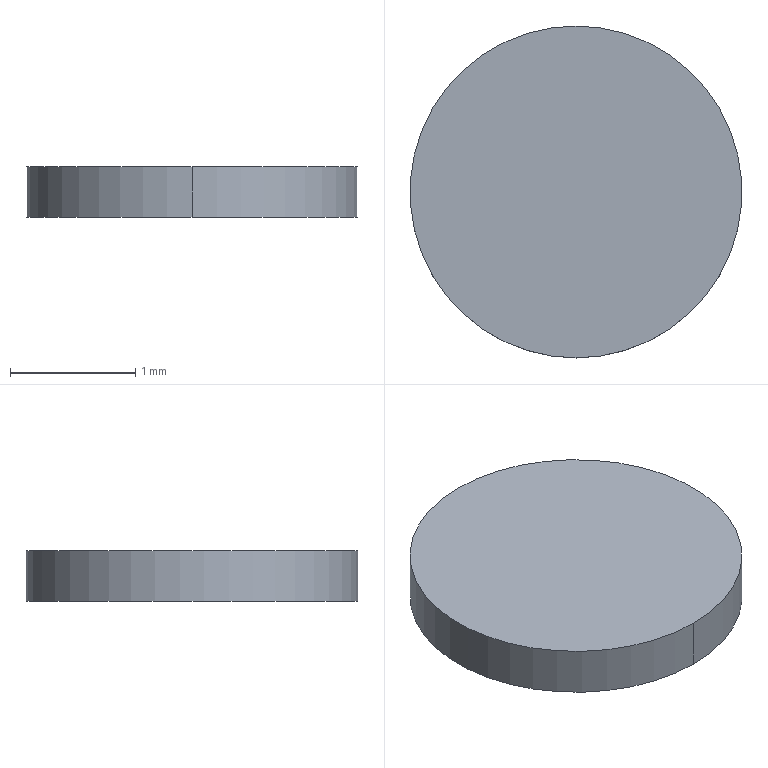Part | STEP file | LRS-150-12_X2_5F00517375-151328 | 1 solid | 4 faces | box 2.65 x 2.65 x 0.4 mm | volume 2.206 mm3 | cylinder 2 | plane 2 | commonest cylinder face diameters 2.65 x2
STEP:
#1=CARTESIAN_POINT('',(0.,0.,0.));
#2=DIRECTION('',(0.,0.,1.));
#3=DIRECTION('',(1.,0.,0.));
#4=AXIS2_PLACEMENT_3D('',#1,#2,#3);
#5=CARTESIAN_POINT('',(-275.667,233.7,-4.8));
#6=VERTEX_POINT('',#5);
#7=CARTESIAN_POINT('',(-275.667,233.7,-4.4));
#8=VERTEX_POINT('',#7);
#9=CARTESIAN_POINT('',(-275.667,233.7,-4.8));
#10=DIRECTION('',(0.,0.,1.));
#11=VECTOR('',#10,1.);
#12=LINE('',#9,#11);
#13=CARTESIAN_POINT('',(-275.667,235.025,-5.145));
#14=DIRECTION('',(0.,0.,-1.));
#15=DIRECTION('',(0.,-1.,0.));
#16=AXIS2_PLACEMENT_3D('',#13,#14,#15);
#17=CYLINDRICAL_SURFACE('',#16,1.325);
#18=CARTESIAN_POINT('',(6.283,-0.345));
#19=DIRECTION('',(0.,-1.));
#20=VECTOR('',#19,1.);
#21=LINE('',#18,#20);
#22=(GEOMETRIC_REPRESENTATION_CONTEXT(2)PARAMETRIC_REPRESENTATION_CONTEXT()REPRESENTATION_CONTEXT('',''));
#23=DEFINITIONAL_REPRESENTATION('',(#21),#22);
#24=PCURVE('',#17,#23);
#25=CARTESIAN_POINT('',(-275.667,235.025,-5.145));
#26=DIRECTION('',(0.,0.,-1.));
#27=DIRECTION('',(0.,-1.,0.));
#28=AXIS2_PLACEMENT_3D('',#25,#26,#27);
#29=CYLINDRICAL_SURFACE('',#28,1.325);
#30=CARTESIAN_POINT('',(0.,-0.345));
#31=DIRECTION('',(0.,-1.));
#32=VECTOR('',#31,1.);
#33=LINE('',#30,#32);
#34=(GEOMETRIC_REPRESENTATION_CONTEXT(2)PARAMETRIC_REPRESENTATION_CONTEXT()REPRESENTATION_CONTEXT('',''));
#35=DEFINITIONAL_REPRESENTATION('',(#33),#34);
#36=PCURVE('',#29,#35);
#37=SURFACE_CURVE('',#12,(#24,#36),.PCURVE_S1.);
#38=EDGE_CURVE('',#6,#8,#37,.T.);
#39=ORIENTED_EDGE('',*,*,#38,.F.);
#40=CARTESIAN_POINT('',(-275.667,236.35,-4.8));
#41=VERTEX_POINT('',#40);
#42=CARTESIAN_POINT('',(-275.667,235.025,-4.8));
#43=DIRECTION('',(0.,0.,-1.));
#44=DIRECTION('',(0.,1.,0.));
#45=AXIS2_PLACEMENT_3D('',#42,#43,#44);
#46=CIRCLE('',#45,1.325);
#47=CARTESIAN_POINT('',(3.142,-0.345));
#48=DIRECTION('',(1.,0.));
#49=VECTOR('',#48,1.);
#50=LINE('',#47,#49);
#51=(GEOMETRIC_REPRESENTATION_CONTEXT(2)PARAMETRIC_REPRESENTATION_CONTEXT()REPRESENTATION_CONTEXT('',''));
#52=DEFINITIONAL_REPRESENTATION('',(#50),#51);
#53=PCURVE('',#17,#52);
#54=CARTESIAN_POINT('',(-217.675,251.825,-4.8));
#55=DIRECTION('',(0.,0.,-1.));
#56=DIRECTION('',(1.,0.,0.));
#57=AXIS2_PLACEMENT_3D('',#54,#55,#56);
#58=PLANE('',#57);
#59=CARTESIAN_POINT('',(-57.991,16.8));
#60=DIRECTION('',(0.,-1.));
#61=AXIS2_PLACEMENT_2D('',#59,#60);
#62=CIRCLE('',#61,1.325);
#63=(GEOMETRIC_REPRESENTATION_CONTEXT(2)PARAMETRIC_REPRESENTATION_CONTEXT()REPRESENTATION_CONTEXT('',''));
#64=DEFINITIONAL_REPRESENTATION('',(#62),#63);
#65=PCURVE('',#58,#64);
#66=SURFACE_CURVE('',#46,(#53,#65),.PCURVE_S1.);
#67=EDGE_CURVE('',#41,#6,#66,.T.);
#68=ORIENTED_EDGE('',*,*,#67,.F.);
#69=CARTESIAN_POINT('',(-275.667,236.35,-4.4));
#70=VERTEX_POINT('',#69);
#71=CARTESIAN_POINT('',(-275.667,236.35,-4.8));
#72=DIRECTION('',(0.,0.,1.));
#73=VECTOR('',#72,1.);
#74=LINE('',#71,#73);
#75=CARTESIAN_POINT('',(3.142,-0.345));
#76=DIRECTION('',(0.,-1.));
#77=VECTOR('',#76,1.);
#78=LINE('',#75,#77);
#79=(GEOMETRIC_REPRESENTATION_CONTEXT(2)PARAMETRIC_REPRESENTATION_CONTEXT()REPRESENTATION_CONTEXT('',''));
#80=DEFINITIONAL_REPRESENTATION('',(#78),#79);
#81=PCURVE('',#17,#80);
#82=CARTESIAN_POINT('',(3.142,-0.345));
#83=DIRECTION('',(0.,-1.));
#84=VECTOR('',#83,1.);
#85=LINE('',#82,#84);
#86=(GEOMETRIC_REPRESENTATION_CONTEXT(2)PARAMETRIC_REPRESENTATION_CONTEXT()REPRESENTATION_CONTEXT('',''));
#87=DEFINITIONAL_REPRESENTATION('',(#85),#86);
#88=PCURVE('',#29,#87);
#89=SURFACE_CURVE('',#74,(#81,#88),.PCURVE_S1.);
#90=EDGE_CURVE('',#41,#70,#89,.T.);
#91=ORIENTED_EDGE('',*,*,#90,.T.);
#92=CARTESIAN_POINT('',(-275.667,235.025,-4.4));
#93=DIRECTION('',(0.,0.,1.));
#94=DIRECTION('',(0.,-1.,0.));
#95=AXIS2_PLACEMENT_3D('',#92,#93,#94);
#96=CIRCLE('',#95,1.325);
#97=CARTESIAN_POINT('',(6.283,-0.745));
#98=DIRECTION('',(-1.,0.));
#99=VECTOR('',#98,1.);
#100=LINE('',#97,#99);
#101=(GEOMETRIC_REPRESENTATION_CONTEXT(2)PARAMETRIC_REPRESENTATION_CONTEXT()REPRESENTATION_CONTEXT('',''));
#102=DEFINITIONAL_REPRESENTATION('',(#100),#101);
#103=PCURVE('',#17,#102);
#104=CARTESIAN_POINT('',(-217.675,251.825,-4.4));
#105=DIRECTION('',(0.,0.,-1.));
#106=DIRECTION('',(1.,0.,0.));
#107=AXIS2_PLACEMENT_3D('',#104,#105,#106);
#108=PLANE('',#107);
#109=CARTESIAN_POINT('',(-57.991,18.125));
#110=CARTESIAN_POINT('',(-55.696,18.125));
#111=CARTESIAN_POINT('',(-56.844,16.137));
#112=CARTESIAN_POINT('',(-57.991,14.15));
#113=CARTESIAN_POINT('',(-59.139,16.137));
#114=CARTESIAN_POINT('',(-60.286,18.125));
#115=CARTESIAN_POINT('',(-57.991,18.125));
#116=(BOUNDED_CURVE()B_SPLINE_CURVE(2,(#109,#110,#111,#112,#113,#114,#115),.UNSPECIFIED.,.T.,.F.)B_SPLINE_CURVE_WITH_KNOTS((1,2,2,2,2,1),(-2.094,0.,2.094,4.189,6.283,8.378),.UNSPECIFIED.)CURVE()GEOMETRIC_REPRESENTATION_ITEM()RATIONAL_B_SPLINE_CURVE((1.,0.5,1.,0.5,1.,0.5,1.))REPRESENTATION_ITEM(''));
#117=(GEOMETRIC_REPRESENTATION_CONTEXT(2)PARAMETRIC_REPRESENTATION_CONTEXT()REPRESENTATION_CONTEXT('',''));
#118=DEFINITIONAL_REPRESENTATION('',(#116),#117);
#119=PCURVE('',#108,#118);
#120=SURFACE_CURVE('',#96,(#103,#119),.PCURVE_S1.);
#121=EDGE_CURVE('',#8,#70,#120,.T.);
#122=ORIENTED_EDGE('',*,*,#121,.F.);
#123=EDGE_LOOP('',(#39,#68,#91,#122));
#124=FACE_BOUND('',#123,.T.);
#125=ADVANCED_FACE('',(#124),#17,.T.);
#126=ORIENTED_EDGE('',*,*,#121,.F.);
#127=CARTESIAN_POINT('',(-275.667,235.025,-4.4));
#128=DIRECTION('',(0.,0.,1.));
#129=DIRECTION('',(0.,1.,0.));
#130=AXIS2_PLACEMENT_3D('',#127,#128,#129);
#131=CIRCLE('',#130,1.325);
#132=CARTESIAN_POINT('',(-57.991,15.475));
#133=CARTESIAN_POINT('',(-60.286,15.475));
#134=CARTESIAN_POINT('',(-59.139,17.462));
#135=CARTESIAN_POINT('',(-57.991,19.45));
#136=CARTESIAN_POINT('',(-56.844,17.462));
#137=CARTESIAN_POINT('',(-55.696,15.475));
#138=CARTESIAN_POINT('',(-57.991,15.475));
#139=(BOUNDED_CURVE()B_SPLINE_CURVE(2,(#132,#133,#134,#135,#136,#137,#138),.UNSPECIFIED.,.T.,.F.)B_SPLINE_CURVE_WITH_KNOTS((1,2,2,2,2,1),(-2.094,0.,2.094,4.189,6.283,8.378),.UNSPECIFIED.)CURVE()GEOMETRIC_REPRESENTATION_ITEM()RATIONAL_B_SPLINE_CURVE((1.,0.5,1.,0.5,1.,0.5,1.))REPRESENTATION_ITEM(''));
#140=(GEOMETRIC_REPRESENTATION_CONTEXT(2)PARAMETRIC_REPRESENTATION_CONTEXT()REPRESENTATION_CONTEXT('',''));
#141=DEFINITIONAL_REPRESENTATION('',(#139),#140);
#142=PCURVE('',#108,#141);
#143=CARTESIAN_POINT('',(3.142,-0.745));
#144=DIRECTION('',(-1.,0.));
#145=VECTOR('',#144,1.);
#146=LINE('',#143,#145);
#147=(GEOMETRIC_REPRESENTATION_CONTEXT(2)PARAMETRIC_REPRESENTATION_CONTEXT()REPRESENTATION_CONTEXT('',''));
#148=DEFINITIONAL_REPRESENTATION('',(#146),#147);
#149=PCURVE('',#29,#148);
#150=SURFACE_CURVE('',#131,(#142,#149),.PCURVE_S1.);
#151=EDGE_CURVE('',#70,#8,#150,.T.);
#152=ORIENTED_EDGE('',*,*,#151,.F.);
#153=EDGE_LOOP('',(#126,#152));
#154=FACE_BOUND('',#153,.F.);
#155=ADVANCED_FACE('',(#154),#108,.F.);
#156=CARTESIAN_POINT('',(-275.667,235.025,-4.8));
#157=DIRECTION('',(0.,0.,-1.));
#158=DIRECTION('',(0.,-1.,0.));
#159=AXIS2_PLACEMENT_3D('',#156,#157,#158);
#160=CIRCLE('',#159,1.325);
#161=CARTESIAN_POINT('',(0.,-0.345));
#162=DIRECTION('',(1.,0.));
#163=VECTOR('',#162,1.);
#164=LINE('',#161,#163);
#165=(GEOMETRIC_REPRESENTATION_CONTEXT(2)PARAMETRIC_REPRESENTATION_CONTEXT()REPRESENTATION_CONTEXT('',''));
#166=DEFINITIONAL_REPRESENTATION('',(#164),#165);
#167=PCURVE('',#29,#166);
#168=CARTESIAN_POINT('',(-57.991,16.8));
#169=DIRECTION('',(0.,1.));
#170=AXIS2_PLACEMENT_2D('',#168,#169);
#171=CIRCLE('',#170,1.325);
#172=(GEOMETRIC_REPRESENTATION_CONTEXT(2)PARAMETRIC_REPRESENTATION_CONTEXT()REPRESENTATION_CONTEXT('',''));
#173=DEFINITIONAL_REPRESENTATION('',(#171),#172);
#174=PCURVE('',#58,#173);
#175=SURFACE_CURVE('',#160,(#167,#174),.PCURVE_S1.);
#176=EDGE_CURVE('',#6,#41,#175,.T.);
#177=ORIENTED_EDGE('',*,*,#176,.F.);
#178=ORIENTED_EDGE('',*,*,#38,.T.);
#179=ORIENTED_EDGE('',*,*,#151,.F.);
#180=ORIENTED_EDGE('',*,*,#90,.F.);
#181=EDGE_LOOP('',(#177,#178,#179,#180));
#182=FACE_BOUND('',#181,.T.);
#183=ADVANCED_FACE('',(#182),#29,.T.);
#184=ORIENTED_EDGE('',*,*,#67,.F.);
#185=ORIENTED_EDGE('',*,*,#176,.F.);
#186=EDGE_LOOP('',(#184,#185));
#187=FACE_BOUND('',#186,.F.);
#188=ADVANCED_FACE('',(#187),#58,.T.);
#189=CLOSED_SHELL('',(#125,#155,#183,#188));
#190=MANIFOLD_SOLID_BREP('',#189);
#191=(LENGTH_UNIT()NAMED_UNIT(*)SI_UNIT(.MILLI.,.METRE.));
#192=UNCERTAINTY_MEASURE_WITH_UNIT(LENGTH_MEASURE(0.0000001),#191,'','');
#193=(NAMED_UNIT(*)PLANE_ANGLE_UNIT()SI_UNIT($,.RADIAN.));
#194=(NAMED_UNIT(*)SI_UNIT($,.STERADIAN.)SOLID_ANGLE_UNIT());
#195=(GEOMETRIC_REPRESENTATION_CONTEXT(3)GLOBAL_UNCERTAINTY_ASSIGNED_CONTEXT((#192))GLOBAL_UNIT_ASSIGNED_CONTEXT((#191,#193,#194))REPRESENTATION_CONTEXT('',''));
#196=ADVANCED_BREP_SHAPE_REPRESENTATION('',(#4,#190),#195);